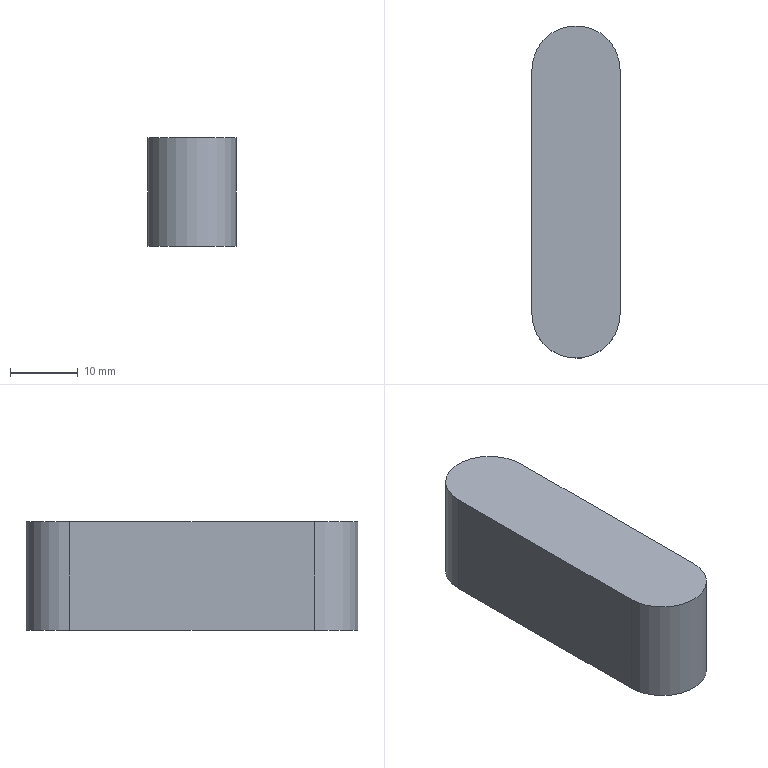Part | NX | features DATUM_CSYS 2, BLEND 1, EXTRUDE 1, OFFSET_REGION 1, SKETCH 1 | 1 solid | 6 faces | box 13 x 49 x 16 mm | volume 9612 mm3 | plane 4 | cylinder 2 | commonest cylinder face diameters 13 x2
STEP:
#1=CARTESIAN_POINT('',(-6.5,18.,16.));
#2=VERTEX_POINT('',#1);
#3=CARTESIAN_POINT('',(-6.5,-18.,16.));
#4=VERTEX_POINT('',#3);
#5=CARTESIAN_POINT('',(-6.5,24.5,16.));
#6=DIRECTION('',(0.,-1.,0.));
#7=VECTOR('',#6,1000.);
#8=LINE('',#5,#7);
#9=EDGE_CURVE('',#2,#4,#8,.T.);
#10=ORIENTED_EDGE('',*,*,#9,.F.);
#11=CARTESIAN_POINT('',(-6.5,18.,0.));
#12=VERTEX_POINT('',#11);
#13=CARTESIAN_POINT('',(-6.5,18.,10.));
#14=DIRECTION('',(0.,0.,-1.));
#15=VECTOR('',#14,1000.);
#16=LINE('',#13,#15);
#17=EDGE_CURVE('',#2,#12,#16,.T.);
#18=ORIENTED_EDGE('',*,*,#17,.T.);
#19=CARTESIAN_POINT('',(-6.5,-18.,0.));
#20=VERTEX_POINT('',#19);
#21=CARTESIAN_POINT('',(-6.5,24.5,0.));
#22=DIRECTION('',(0.,-1.,0.));
#23=VECTOR('',#22,1000.);
#24=LINE('',#21,#23);
#25=EDGE_CURVE('',#12,#20,#24,.T.);
#26=ORIENTED_EDGE('',*,*,#25,.T.);
#27=CARTESIAN_POINT('',(-6.5,-18.,10.));
#28=DIRECTION('',(0.,0.,-1.));
#29=VECTOR('',#28,1000.);
#30=LINE('',#27,#29);
#31=EDGE_CURVE('',#20,#4,#30,.F.);
#32=ORIENTED_EDGE('',*,*,#31,.T.);
#33=EDGE_LOOP('',(#10,#18,#26,#32));
#34=FACE_BOUND('',#33,.T.);
#35=CARTESIAN_POINT('',(-6.5,24.5,10.));
#36=DIRECTION('',(1.,0.,0.));
#37=DIRECTION('',(0.,0.,-1.));
#38=AXIS2_PLACEMENT_3D('',#35,#36,#37);
#39=PLANE('',#38);
#40=ADVANCED_FACE('',(#34),#39,.F.);
#41=CARTESIAN_POINT('',(6.5,-18.,0.));
#42=VERTEX_POINT('',#41);
#43=CARTESIAN_POINT('',(6.5,18.,0.));
#44=VERTEX_POINT('',#43);
#45=CARTESIAN_POINT('',(6.5,-24.5,0.));
#46=DIRECTION('',(0.,1.,0.));
#47=VECTOR('',#46,1000.);
#48=LINE('',#45,#47);
#49=EDGE_CURVE('',#42,#44,#48,.T.);
#50=ORIENTED_EDGE('',*,*,#49,.T.);
#51=CARTESIAN_POINT('',(6.5,18.,16.));
#52=VERTEX_POINT('',#51);
#53=CARTESIAN_POINT('',(6.5,18.,10.));
#54=DIRECTION('',(0.,0.,-1.));
#55=VECTOR('',#54,1000.);
#56=LINE('',#53,#55);
#57=EDGE_CURVE('',#44,#52,#56,.F.);
#58=ORIENTED_EDGE('',*,*,#57,.T.);
#59=CARTESIAN_POINT('',(6.5,-18.,16.));
#60=VERTEX_POINT('',#59);
#61=CARTESIAN_POINT('',(6.5,-24.5,16.));
#62=DIRECTION('',(0.,1.,0.));
#63=VECTOR('',#62,1000.);
#64=LINE('',#61,#63);
#65=EDGE_CURVE('',#60,#52,#64,.T.);
#66=ORIENTED_EDGE('',*,*,#65,.F.);
#67=CARTESIAN_POINT('',(6.5,-18.,10.));
#68=DIRECTION('',(0.,0.,-1.));
#69=VECTOR('',#68,1000.);
#70=LINE('',#67,#69);
#71=EDGE_CURVE('',#60,#42,#70,.T.);
#72=ORIENTED_EDGE('',*,*,#71,.T.);
#73=EDGE_LOOP('',(#50,#58,#66,#72));
#74=FACE_BOUND('',#73,.T.);
#75=CARTESIAN_POINT('',(6.5,-24.5,10.));
#76=DIRECTION('',(-1.,0.,0.));
#77=DIRECTION('',(0.,0.,1.));
#78=AXIS2_PLACEMENT_3D('',#75,#76,#77);
#79=PLANE('',#78);
#80=ADVANCED_FACE('',(#74),#79,.F.);
#81=CARTESIAN_POINT('',(0.,18.,16.));
#82=DIRECTION('',(0.,0.,1.));
#83=DIRECTION('',(1.,0.,0.));
#84=AXIS2_PLACEMENT_3D('',#81,#82,#83);
#85=CIRCLE('',#84,6.5);
#86=EDGE_CURVE('',#52,#2,#85,.T.);
#87=ORIENTED_EDGE('',*,*,#86,.T.);
#88=ORIENTED_EDGE('',*,*,#9,.T.);
#89=CARTESIAN_POINT('',(0.,-18.,16.));
#90=DIRECTION('',(0.,0.,1.));
#91=DIRECTION('',(1.,0.,0.));
#92=AXIS2_PLACEMENT_3D('',#89,#90,#91);
#93=CIRCLE('',#92,6.5);
#94=EDGE_CURVE('',#4,#60,#93,.T.);
#95=ORIENTED_EDGE('',*,*,#94,.T.);
#96=ORIENTED_EDGE('',*,*,#65,.T.);
#97=EDGE_LOOP('',(#87,#88,#95,#96));
#98=FACE_BOUND('',#97,.T.);
#99=CARTESIAN_POINT('',(0.,0.,16.));
#100=DIRECTION('',(0.,0.,1.));
#101=DIRECTION('',(1.,0.,0.));
#102=AXIS2_PLACEMENT_3D('',#99,#100,#101);
#103=PLANE('',#102);
#104=ADVANCED_FACE('',(#98),#103,.T.);
#105=ORIENTED_EDGE('',*,*,#25,.F.);
#106=CARTESIAN_POINT('',(0.,18.,0.));
#107=DIRECTION('',(0.,0.,1.));
#108=DIRECTION('',(1.,0.,0.));
#109=AXIS2_PLACEMENT_3D('',#106,#107,#108);
#110=CIRCLE('',#109,6.5);
#111=EDGE_CURVE('',#12,#44,#110,.F.);
#112=ORIENTED_EDGE('',*,*,#111,.T.);
#113=ORIENTED_EDGE('',*,*,#49,.F.);
#114=CARTESIAN_POINT('',(0.,-18.,0.));
#115=DIRECTION('',(0.,0.,1.));
#116=DIRECTION('',(1.,0.,0.));
#117=AXIS2_PLACEMENT_3D('',#114,#115,#116);
#118=CIRCLE('',#117,6.5);
#119=EDGE_CURVE('',#42,#20,#118,.F.);
#120=ORIENTED_EDGE('',*,*,#119,.T.);
#121=EDGE_LOOP('',(#105,#112,#113,#120));
#122=FACE_BOUND('',#121,.T.);
#123=CARTESIAN_POINT('',(0.,0.,0.));
#124=DIRECTION('',(0.,0.,1.));
#125=DIRECTION('',(1.,0.,0.));
#126=AXIS2_PLACEMENT_3D('',#123,#124,#125);
#127=PLANE('',#126);
#128=ADVANCED_FACE('',(#122),#127,.F.);
#129=ORIENTED_EDGE('',*,*,#111,.F.);
#130=ORIENTED_EDGE('',*,*,#17,.F.);
#131=ORIENTED_EDGE('',*,*,#86,.F.);
#132=ORIENTED_EDGE('',*,*,#57,.F.);
#133=EDGE_LOOP('',(#129,#130,#131,#132));
#134=FACE_BOUND('',#133,.T.);
#135=CARTESIAN_POINT('',(0.,18.,10.));
#136=DIRECTION('',(0.,0.,-1.));
#137=DIRECTION('',(-1.,0.,0.));
#138=AXIS2_PLACEMENT_3D('',#135,#136,#137);
#139=CYLINDRICAL_SURFACE('',#138,6.5);
#140=ADVANCED_FACE('',(#134),#139,.T.);
#141=ORIENTED_EDGE('',*,*,#71,.F.);
#142=ORIENTED_EDGE('',*,*,#94,.F.);
#143=ORIENTED_EDGE('',*,*,#31,.F.);
#144=ORIENTED_EDGE('',*,*,#119,.F.);
#145=EDGE_LOOP('',(#141,#142,#143,#144));
#146=FACE_BOUND('',#145,.T.);
#147=CARTESIAN_POINT('',(0.,-18.,10.));
#148=DIRECTION('',(0.,0.,-1.));
#149=DIRECTION('',(-1.,0.,0.));
#150=AXIS2_PLACEMENT_3D('',#147,#148,#149);
#151=CYLINDRICAL_SURFACE('',#150,6.5);
#152=ADVANCED_FACE('',(#146),#151,.T.);
#153=CLOSED_SHELL('',(#40,#80,#104,#128,#140,#152));
#154=MANIFOLD_SOLID_BREP('',#153);
#155=(LENGTH_UNIT()NAMED_UNIT(*)SI_UNIT(.MILLI.,.METRE.));
#156=UNCERTAINTY_MEASURE_WITH_UNIT(LENGTH_MEASURE(0.00001),#155,'','');
#157=(NAMED_UNIT(*)PLANE_ANGLE_UNIT()SI_UNIT($,.RADIAN.));
#158=(NAMED_UNIT(*)SI_UNIT($,.STERADIAN.)SOLID_ANGLE_UNIT());
#159=(GEOMETRIC_REPRESENTATION_CONTEXT(3)GLOBAL_UNCERTAINTY_ASSIGNED_CONTEXT((#156))GLOBAL_UNIT_ASSIGNED_CONTEXT((#155,#157,#158))REPRESENTATION_CONTEXT('',''));
#160=ADVANCED_BREP_SHAPE_REPRESENTATION('',(#154),#159);